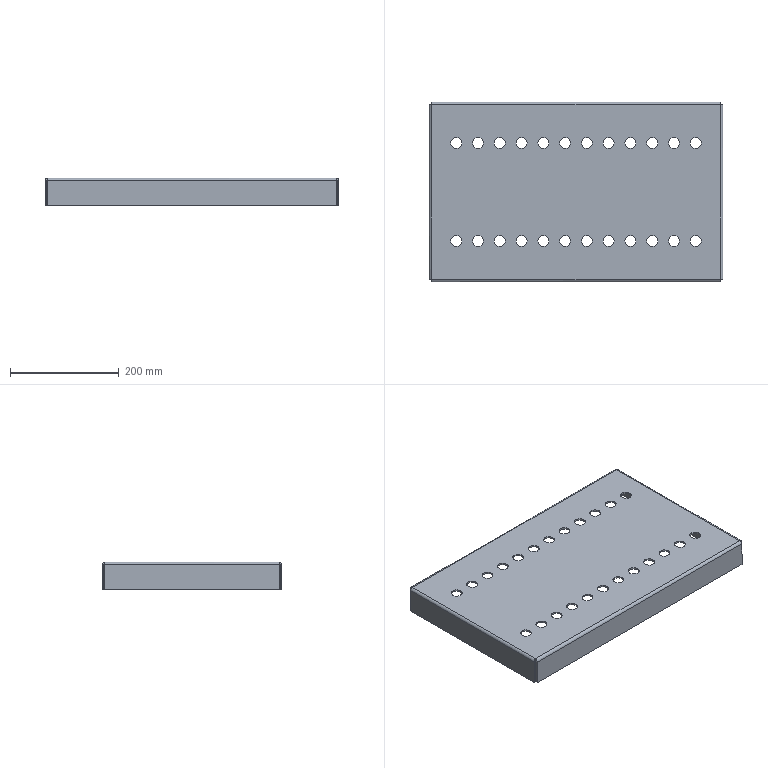Part | STEP file | Produce dryer line heating fan-OVEN-451 | 1 solid | 86 faces | box 540 x 330 x 51 mm | volume 750332 mm3 | cylinder 56 | plane 22 | spline 8 | commonest cylinder face diameters 20 x48 4 x4 10 x4